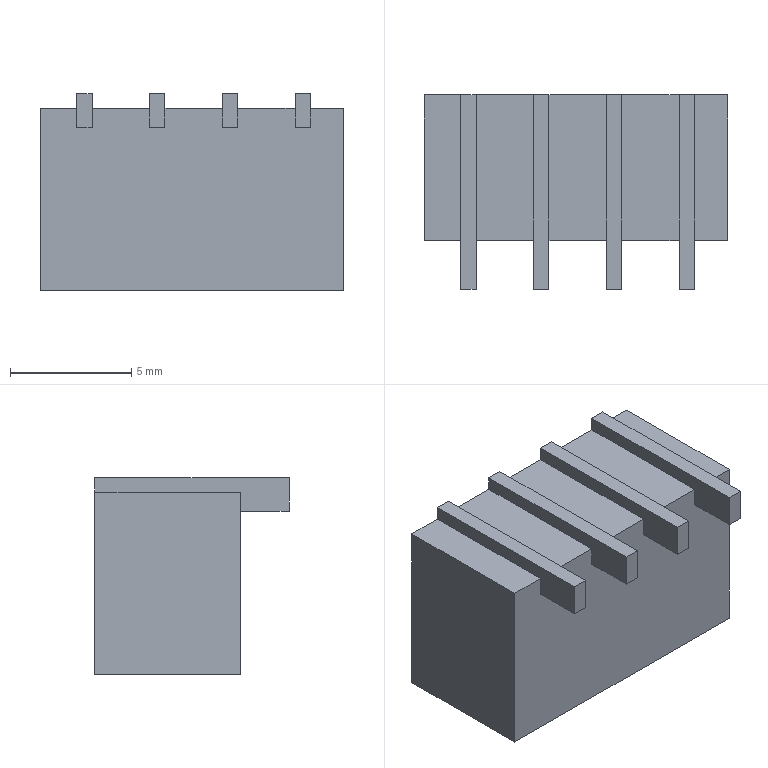Part | SolidWorks | features Boss 1, Cut 1, Extrusion 1 | 1 solid | 47 faces | box 12.5 x 8 x 8.081 mm | volume 341.66 mm3 | plane 39 | cylinder 8 | commonest cylinder face diameters 0.961 x2 1.001 x2 1.034 x2 1.165 x2
STEP:
#1=CARTESIAN_POINT('',(1.73,2.192,5.));
#2=VERTEX_POINT('',#1);
#3=CARTESIAN_POINT('',(2.731,2.192,5.));
#4=VERTEX_POINT('',#3);
#5=CARTESIAN_POINT('',(2.231,2.192,5.));
#6=DIRECTION('',(0.,0.,-1.));
#7=DIRECTION('',(-1.,0.,0.));
#8=AXIS2_PLACEMENT_3D('',#5,#6,#7);
#9=CIRCLE('',#8,0.5005);
#10=EDGE_CURVE('',#2,#4,#9,.T.);
#11=ORIENTED_EDGE('',*,*,#10,.T.);
#12=CARTESIAN_POINT('',(2.731,2.192,0.));
#13=VERTEX_POINT('',#12);
#14=CARTESIAN_POINT('',(2.731,2.192,5.));
#15=DIRECTION('',(0.,0.,-1.));
#16=VECTOR('',#15,1000.);
#17=LINE('',#14,#16);
#18=EDGE_CURVE('',#4,#13,#17,.T.);
#19=ORIENTED_EDGE('',*,*,#18,.T.);
#20=CARTESIAN_POINT('',(1.73,2.192,0.));
#21=VERTEX_POINT('',#20);
#22=CARTESIAN_POINT('',(2.231,2.192,0.));
#23=DIRECTION('',(0.,0.,-1.));
#24=DIRECTION('',(-1.,0.,0.));
#25=AXIS2_PLACEMENT_3D('',#22,#23,#24);
#26=CIRCLE('',#25,0.5005);
#27=EDGE_CURVE('',#21,#13,#26,.T.);
#28=ORIENTED_EDGE('',*,*,#27,.F.);
#29=CARTESIAN_POINT('',(1.73,2.192,5.));
#30=DIRECTION('',(0.,0.,-1.));
#31=VECTOR('',#30,1000.);
#32=LINE('',#29,#31);
#33=EDGE_CURVE('',#2,#21,#32,.T.);
#34=ORIENTED_EDGE('',*,*,#33,.F.);
#35=EDGE_LOOP('',(#11,#19,#28,#34));
#36=FACE_OUTER_BOUND('',#35,.T.);
#37=CARTESIAN_POINT('',(2.231,2.192,5.));
#38=DIRECTION('',(0.,0.,-1.));
#39=DIRECTION('',(-1.,0.,0.));
#40=AXIS2_PLACEMENT_3D('',#37,#38,#39);
#41=CYLINDRICAL_SURFACE('',#40,0.5005);
#42=ADVANCED_FACE('',(#36),#41,.T.);
#43=CARTESIAN_POINT('',(3.717,2.192,5.));
#44=VERTEX_POINT('',#43);
#45=CARTESIAN_POINT('',(4.882,2.192,5.));
#46=VERTEX_POINT('',#45);
#47=CARTESIAN_POINT('',(4.299,2.192,5.));
#48=DIRECTION('',(0.,0.,-1.));
#49=DIRECTION('',(-1.,0.,0.));
#50=AXIS2_PLACEMENT_3D('',#47,#48,#49);
#51=CIRCLE('',#50,0.5827);
#52=EDGE_CURVE('',#44,#46,#51,.T.);
#53=ORIENTED_EDGE('',*,*,#52,.T.);
#54=CARTESIAN_POINT('',(4.882,2.192,0.));
#55=VERTEX_POINT('',#54);
#56=CARTESIAN_POINT('',(4.882,2.192,5.));
#57=DIRECTION('',(0.,0.,-1.));
#58=VECTOR('',#57,1000.);
#59=LINE('',#56,#58);
#60=EDGE_CURVE('',#46,#55,#59,.T.);
#61=ORIENTED_EDGE('',*,*,#60,.T.);
#62=CARTESIAN_POINT('',(3.717,2.192,0.));
#63=VERTEX_POINT('',#62);
#64=CARTESIAN_POINT('',(4.299,2.192,0.));
#65=DIRECTION('',(0.,0.,-1.));
#66=DIRECTION('',(-1.,0.,0.));
#67=AXIS2_PLACEMENT_3D('',#64,#65,#66);
#68=CIRCLE('',#67,0.5827);
#69=EDGE_CURVE('',#63,#55,#68,.T.);
#70=ORIENTED_EDGE('',*,*,#69,.F.);
#71=CARTESIAN_POINT('',(3.717,2.192,5.));
#72=DIRECTION('',(0.,0.,-1.));
#73=VECTOR('',#72,1000.);
#74=LINE('',#71,#73);
#75=EDGE_CURVE('',#44,#63,#74,.T.);
#76=ORIENTED_EDGE('',*,*,#75,.F.);
#77=EDGE_LOOP('',(#53,#61,#70,#76));
#78=FACE_OUTER_BOUND('',#77,.T.);
#79=CARTESIAN_POINT('',(4.299,2.192,5.));
#80=DIRECTION('',(0.,0.,-1.));
#81=DIRECTION('',(-1.,0.,0.));
#82=AXIS2_PLACEMENT_3D('',#79,#80,#81);
#83=CYLINDRICAL_SURFACE('',#82,0.5827);
#84=ADVANCED_FACE('',(#78),#83,.T.);
#85=CARTESIAN_POINT('',(5.817,2.192,5.));
#86=VERTEX_POINT('',#85);
#87=CARTESIAN_POINT('',(6.852,2.192,5.));
#88=VERTEX_POINT('',#87);
#89=CARTESIAN_POINT('',(6.335,2.192,5.));
#90=DIRECTION('',(0.,0.,-1.));
#91=DIRECTION('',(-1.,0.,0.));
#92=AXIS2_PLACEMENT_3D('',#89,#90,#91);
#93=CIRCLE('',#92,0.5172);
#94=EDGE_CURVE('',#86,#88,#93,.T.);
#95=ORIENTED_EDGE('',*,*,#94,.T.);
#96=CARTESIAN_POINT('',(6.852,2.192,0.));
#97=VERTEX_POINT('',#96);
#98=CARTESIAN_POINT('',(6.852,2.192,5.));
#99=DIRECTION('',(0.,0.,-1.));
#100=VECTOR('',#99,1000.);
#101=LINE('',#98,#100);
#102=EDGE_CURVE('',#88,#97,#101,.T.);
#103=ORIENTED_EDGE('',*,*,#102,.T.);
#104=CARTESIAN_POINT('',(5.817,2.192,0.));
#105=VERTEX_POINT('',#104);
#106=CARTESIAN_POINT('',(6.335,2.192,0.));
#107=DIRECTION('',(0.,0.,-1.));
#108=DIRECTION('',(-1.,0.,0.));
#109=AXIS2_PLACEMENT_3D('',#106,#107,#108);
#110=CIRCLE('',#109,0.5172);
#111=EDGE_CURVE('',#105,#97,#110,.T.);
#112=ORIENTED_EDGE('',*,*,#111,.F.);
#113=CARTESIAN_POINT('',(5.817,2.192,5.));
#114=DIRECTION('',(0.,0.,-1.));
#115=VECTOR('',#114,1000.);
#116=LINE('',#113,#115);
#117=EDGE_CURVE('',#86,#105,#116,.T.);
#118=ORIENTED_EDGE('',*,*,#117,.F.);
#119=EDGE_LOOP('',(#95,#103,#112,#118));
#120=FACE_OUTER_BOUND('',#119,.T.);
#121=CARTESIAN_POINT('',(6.335,2.192,5.));
#122=DIRECTION('',(0.,0.,-1.));
#123=DIRECTION('',(-1.,0.,0.));
#124=AXIS2_PLACEMENT_3D('',#121,#122,#123);
#125=CYLINDRICAL_SURFACE('',#124,0.5172);
#126=ADVANCED_FACE('',(#120),#125,.T.);
#127=CARTESIAN_POINT('',(7.506,2.192,5.));
#128=VERTEX_POINT('',#127);
#129=CARTESIAN_POINT('',(8.467,2.192,5.));
#130=VERTEX_POINT('',#129);
#131=CARTESIAN_POINT('',(7.986,2.192,5.));
#132=DIRECTION('',(0.,0.,-1.));
#133=DIRECTION('',(-1.,0.,0.));
#134=AXIS2_PLACEMENT_3D('',#131,#132,#133);
#135=CIRCLE('',#134,0.4804);
#136=EDGE_CURVE('',#128,#130,#135,.T.);
#137=ORIENTED_EDGE('',*,*,#136,.T.);
#138=CARTESIAN_POINT('',(8.467,2.192,0.));
#139=VERTEX_POINT('',#138);
#140=CARTESIAN_POINT('',(8.467,2.192,5.));
#141=DIRECTION('',(0.,0.,-1.));
#142=VECTOR('',#141,1000.);
#143=LINE('',#140,#142);
#144=EDGE_CURVE('',#130,#139,#143,.T.);
#145=ORIENTED_EDGE('',*,*,#144,.T.);
#146=CARTESIAN_POINT('',(7.506,2.192,0.));
#147=VERTEX_POINT('',#146);
#148=CARTESIAN_POINT('',(7.986,2.192,0.));
#149=DIRECTION('',(0.,0.,-1.));
#150=DIRECTION('',(-1.,0.,0.));
#151=AXIS2_PLACEMENT_3D('',#148,#149,#150);
#152=CIRCLE('',#151,0.4804);
#153=EDGE_CURVE('',#147,#139,#152,.T.);
#154=ORIENTED_EDGE('',*,*,#153,.F.);
#155=CARTESIAN_POINT('',(7.506,2.192,5.));
#156=DIRECTION('',(0.,0.,-1.));
#157=VECTOR('',#156,1000.);
#158=LINE('',#155,#157);
#159=EDGE_CURVE('',#128,#147,#158,.T.);
#160=ORIENTED_EDGE('',*,*,#159,.F.);
#161=EDGE_LOOP('',(#137,#145,#154,#160));
#162=FACE_OUTER_BOUND('',#161,.T.);
#163=CARTESIAN_POINT('',(7.986,2.192,5.));
#164=DIRECTION('',(0.,0.,-1.));
#165=DIRECTION('',(-1.,0.,0.));
#166=AXIS2_PLACEMENT_3D('',#163,#164,#165);
#167=CYLINDRICAL_SURFACE('',#166,0.4804);
#168=ADVANCED_FACE('',(#162),#167,.T.);
#169=CARTESIAN_POINT('',(0.9207,-1.386,6.717));
#170=VERTEX_POINT('',#169);
#171=CARTESIAN_POINT('',(0.9207,-1.386,7.5));
#172=VERTEX_POINT('',#171);
#173=CARTESIAN_POINT('',(0.9207,-1.386,7.5));
#174=DIRECTION('',(0.,0.,1.));
#175=VECTOR('',#174,1000.);
#176=LINE('',#173,#175);
#177=EDGE_CURVE('',#170,#172,#176,.T.);
#178=ORIENTED_EDGE('',*,*,#177,.F.);
#179=CARTESIAN_POINT('',(0.2773,-1.386,6.717));
#180=VERTEX_POINT('',#179);
#181=CARTESIAN_POINT('',(11.283,-1.386,6.717));
#182=DIRECTION('',(1.,0.,0.));
#183=VECTOR('',#182,1000.);
#184=LINE('',#181,#183);
#185=EDGE_CURVE('',#180,#170,#184,.T.);
#186=ORIENTED_EDGE('',*,*,#185,.F.);
#187=CARTESIAN_POINT('',(0.2773,-1.386,7.5));
#188=VERTEX_POINT('',#187);
#189=CARTESIAN_POINT('',(0.2773,-1.386,7.5));
#190=DIRECTION('',(0.,0.,-1.));
#191=VECTOR('',#190,1000.);
#192=LINE('',#189,#191);
#193=EDGE_CURVE('',#188,#180,#192,.T.);
#194=ORIENTED_EDGE('',*,*,#193,.F.);
#195=CARTESIAN_POINT('',(-1.217,-1.386,7.5));
#196=VERTEX_POINT('',#195);
#197=CARTESIAN_POINT('',(11.283,-1.386,7.5));
#198=DIRECTION('',(1.,0.,0.));
#199=VECTOR('',#198,1000.);
#200=LINE('',#197,#199);
#201=EDGE_CURVE('',#196,#188,#200,.T.);
#202=ORIENTED_EDGE('',*,*,#201,.F.);
#203=CARTESIAN_POINT('',(-1.217,-1.386,0.));
#204=VERTEX_POINT('',#203);
#205=CARTESIAN_POINT('',(-1.217,-1.386,7.5));
#206=DIRECTION('',(0.,0.,-1.));
#207=VECTOR('',#206,1000.);
#208=LINE('',#205,#207);
#209=EDGE_CURVE('',#196,#204,#208,.T.);
#210=ORIENTED_EDGE('',*,*,#209,.T.);
#211=CARTESIAN_POINT('',(11.283,-1.386,0.));
#212=VERTEX_POINT('',#211);
#213=CARTESIAN_POINT('',(11.283,-1.386,0.));
#214=DIRECTION('',(1.,0.,0.));
#215=VECTOR('',#214,1000.);
#216=LINE('',#213,#215);
#217=EDGE_CURVE('',#204,#212,#216,.T.);
#218=ORIENTED_EDGE('',*,*,#217,.T.);
#219=CARTESIAN_POINT('',(11.283,-1.386,7.5));
#220=VERTEX_POINT('',#219);
#221=CARTESIAN_POINT('',(11.283,-1.386,7.5));
#222=DIRECTION('',(0.,0.,-1.));
#223=VECTOR('',#222,1000.);
#224=LINE('',#221,#223);
#225=EDGE_CURVE('',#220,#212,#224,.T.);
#226=ORIENTED_EDGE('',*,*,#225,.F.);
#227=CARTESIAN_POINT('',(9.921,-1.386,7.5));
#228=VERTEX_POINT('',#227);
#229=CARTESIAN_POINT('',(11.283,-1.386,7.5));
#230=DIRECTION('',(1.,0.,0.));
#231=VECTOR('',#230,1000.);
#232=LINE('',#229,#231);
#233=EDGE_CURVE('',#228,#220,#232,.T.);
#234=ORIENTED_EDGE('',*,*,#233,.F.);
#235=CARTESIAN_POINT('',(9.921,-1.386,6.717));
#236=VERTEX_POINT('',#235);
#237=CARTESIAN_POINT('',(9.921,-1.386,7.5));
#238=DIRECTION('',(0.,0.,1.));
#239=VECTOR('',#238,1000.);
#240=LINE('',#237,#239);
#241=EDGE_CURVE('',#236,#228,#240,.T.);
#242=ORIENTED_EDGE('',*,*,#241,.F.);
#243=CARTESIAN_POINT('',(9.277,-1.386,6.717));
#244=VERTEX_POINT('',#243);
#245=CARTESIAN_POINT('',(11.283,-1.386,6.717));
#246=DIRECTION('',(1.,0.,0.));
#247=VECTOR('',#246,1000.);
#248=LINE('',#245,#247);
#249=EDGE_CURVE('',#244,#236,#248,.T.);
#250=ORIENTED_EDGE('',*,*,#249,.F.);
#251=CARTESIAN_POINT('',(9.277,-1.386,7.5));
#252=VERTEX_POINT('',#251);
#253=CARTESIAN_POINT('',(9.277,-1.386,7.5));
#254=DIRECTION('',(0.,0.,-1.));
#255=VECTOR('',#254,1000.);
#256=LINE('',#253,#255);
#257=EDGE_CURVE('',#252,#244,#256,.T.);
#258=ORIENTED_EDGE('',*,*,#257,.F.);
#259=CARTESIAN_POINT('',(6.921,-1.386,7.5));
#260=VERTEX_POINT('',#259);
#261=CARTESIAN_POINT('',(11.283,-1.386,7.5));
#262=DIRECTION('',(1.,0.,0.));
#263=VECTOR('',#262,1000.);
#264=LINE('',#261,#263);
#265=EDGE_CURVE('',#260,#252,#264,.T.);
#266=ORIENTED_EDGE('',*,*,#265,.F.);
#267=CARTESIAN_POINT('',(6.921,-1.386,6.717));
#268=VERTEX_POINT('',#267);
#269=CARTESIAN_POINT('',(6.921,-1.386,7.5));
#270=DIRECTION('',(0.,0.,1.));
#271=VECTOR('',#270,1000.);
#272=LINE('',#269,#271);
#273=EDGE_CURVE('',#268,#260,#272,.T.);
#274=ORIENTED_EDGE('',*,*,#273,.F.);
#275=CARTESIAN_POINT('',(6.277,-1.386,6.717));
#276=VERTEX_POINT('',#275);
#277=CARTESIAN_POINT('',(11.283,-1.386,6.717));
#278=DIRECTION('',(1.,0.,0.));
#279=VECTOR('',#278,1000.);
#280=LINE('',#277,#279);
#281=EDGE_CURVE('',#276,#268,#280,.T.);
#282=ORIENTED_EDGE('',*,*,#281,.F.);
#283=CARTESIAN_POINT('',(6.277,-1.386,7.5));
#284=VERTEX_POINT('',#283);
#285=CARTESIAN_POINT('',(6.277,-1.386,7.5));
#286=DIRECTION('',(0.,0.,-1.));
#287=VECTOR('',#286,1000.);
#288=LINE('',#285,#287);
#289=EDGE_CURVE('',#284,#276,#288,.T.);
#290=ORIENTED_EDGE('',*,*,#289,.F.);
#291=CARTESIAN_POINT('',(3.921,-1.386,7.5));
#292=VERTEX_POINT('',#291);
#293=CARTESIAN_POINT('',(11.283,-1.386,7.5));
#294=DIRECTION('',(1.,0.,0.));
#295=VECTOR('',#294,1000.);
#296=LINE('',#293,#295);
#297=EDGE_CURVE('',#292,#284,#296,.T.);
#298=ORIENTED_EDGE('',*,*,#297,.F.);
#299=CARTESIAN_POINT('',(3.921,-1.386,6.717));
#300=VERTEX_POINT('',#299);
#301=CARTESIAN_POINT('',(3.921,-1.386,7.5));
#302=DIRECTION('',(0.,0.,1.));
#303=VECTOR('',#302,1000.);
#304=LINE('',#301,#303);
#305=EDGE_CURVE('',#300,#292,#304,.T.);
#306=ORIENTED_EDGE('',*,*,#305,.F.);
#307=CARTESIAN_POINT('',(3.277,-1.386,6.717));
#308=VERTEX_POINT('',#307);
#309=CARTESIAN_POINT('',(11.283,-1.386,6.717));
#310=DIRECTION('',(1.,0.,0.));
#311=VECTOR('',#310,1000.);
#312=LINE('',#309,#311);
#313=EDGE_CURVE('',#308,#300,#312,.T.);
#314=ORIENTED_EDGE('',*,*,#313,.F.);
#315=CARTESIAN_POINT('',(3.277,-1.386,7.5));
#316=VERTEX_POINT('',#315);
#317=CARTESIAN_POINT('',(3.277,-1.386,7.5));
#318=DIRECTION('',(0.,0.,-1.));
#319=VECTOR('',#318,1000.);
#320=LINE('',#317,#319);
#321=EDGE_CURVE('',#316,#308,#320,.T.);
#322=ORIENTED_EDGE('',*,*,#321,.F.);
#323=CARTESIAN_POINT('',(11.283,-1.386,7.5));
#324=DIRECTION('',(1.,0.,0.));
#325=VECTOR('',#324,1000.);
#326=LINE('',#323,#325);
#327=EDGE_CURVE('',#172,#316,#326,.T.);
#328=ORIENTED_EDGE('',*,*,#327,.F.);
#329=EDGE_LOOP('',(#178,#186,#194,#202,#210,#218,#226,#234,#242,#250,#258,#266,#274,#282,#290,#298,#306,#314,#322,#328));
#330=FACE_OUTER_BOUND('',#329,.T.);
#331=CARTESIAN_POINT('',(11.283,-1.386,7.5));
#332=DIRECTION('',(0.,1.,0.));
#333=DIRECTION('',(-1.,0.,0.));
#334=AXIS2_PLACEMENT_3D('',#331,#332,#333);
#335=PLANE('',#334);
#336=ADVANCED_FACE('',(#330),#335,.F.);
#337=CARTESIAN_POINT('',(3.277,4.614,7.5));
#338=VERTEX_POINT('',#337);
#339=CARTESIAN_POINT('',(0.9207,4.614,7.5));
#340=VERTEX_POINT('',#339);
#341=CARTESIAN_POINT('',(11.283,4.614,7.5));
#342=DIRECTION('',(-1.,0.,0.));
#343=VECTOR('',#342,1000.);
#344=LINE('',#341,#343);
#345=EDGE_CURVE('',#338,#340,#344,.T.);
#346=ORIENTED_EDGE('',*,*,#345,.T.);
#347=CARTESIAN_POINT('',(0.9207,4.614,7.5));
#348=DIRECTION('',(0.,-1.,0.));
#349=VECTOR('',#348,1000.);
#350=LINE('',#347,#349);
#351=EDGE_CURVE('',#340,#172,#350,.T.);
#352=ORIENTED_EDGE('',*,*,#351,.T.);
#353=ORIENTED_EDGE('',*,*,#327,.T.);
#354=CARTESIAN_POINT('',(3.277,4.614,7.5));
#355=DIRECTION('',(0.,1.,0.));
#356=VECTOR('',#355,1000.);
#357=LINE('',#354,#356);
#358=EDGE_CURVE('',#316,#338,#357,.T.);
#359=ORIENTED_EDGE('',*,*,#358,.T.);
#360=EDGE_LOOP('',(#346,#352,#353,#359));
#361=FACE_OUTER_BOUND('',#360,.T.);
#362=CARTESIAN_POINT('',(11.283,4.614,7.5));
#363=DIRECTION('',(0.,0.,1.));
#364=DIRECTION('',(1.,0.,0.));
#365=AXIS2_PLACEMENT_3D('',#362,#363,#364);
#366=PLANE('',#365);
#367=ADVANCED_FACE('',(#361),#366,.T.);
#368=ORIENTED_EDGE('',*,*,#201,.T.);
#369=CARTESIAN_POINT('',(0.2773,4.614,7.5));
#370=VERTEX_POINT('',#369);
#371=CARTESIAN_POINT('',(0.2773,4.614,7.5));
#372=DIRECTION('',(0.,1.,0.));
#373=VECTOR('',#372,1000.);
#374=LINE('',#371,#373);
#375=EDGE_CURVE('',#188,#370,#374,.T.);
#376=ORIENTED_EDGE('',*,*,#375,.T.);
#377=CARTESIAN_POINT('',(-1.217,4.614,7.5));
#378=VERTEX_POINT('',#377);
#379=CARTESIAN_POINT('',(11.283,4.614,7.5));
#380=DIRECTION('',(-1.,0.,0.));
#381=VECTOR('',#380,1000.);
#382=LINE('',#379,#381);
#383=EDGE_CURVE('',#370,#378,#382,.T.);
#384=ORIENTED_EDGE('',*,*,#383,.T.);
#385=CARTESIAN_POINT('',(-1.217,-1.386,7.5));
#386=DIRECTION('',(0.,-1.,0.));
#387=VECTOR('',#386,1000.);
#388=LINE('',#385,#387);
#389=EDGE_CURVE('',#378,#196,#388,.T.);
#390=ORIENTED_EDGE('',*,*,#389,.T.);
#391=EDGE_LOOP('',(#368,#376,#384,#390));
#392=FACE_OUTER_BOUND('',#391,.T.);
#393=CARTESIAN_POINT('',(11.283,4.614,7.5));
#394=DIRECTION('',(0.,0.,1.));
#395=DIRECTION('',(1.,0.,0.));
#396=AXIS2_PLACEMENT_3D('',#393,#394,#395);
#397=PLANE('',#396);
#398=ADVANCED_FACE('',(#392),#397,.T.);
#399=CARTESIAN_POINT('',(6.277,4.614,7.5));
#400=VERTEX_POINT('',#399);
#401=CARTESIAN_POINT('',(3.921,4.614,7.5));
#402=VERTEX_POINT('',#401);
#403=CARTESIAN_POINT('',(11.283,4.614,7.5));
#404=DIRECTION('',(-1.,0.,0.));
#405=VECTOR('',#404,1000.);
#406=LINE('',#403,#405);
#407=EDGE_CURVE('',#400,#402,#406,.T.);
#408=ORIENTED_EDGE('',*,*,#407,.T.);
#409=CARTESIAN_POINT('',(3.921,4.614,7.5));
#410=DIRECTION('',(0.,-1.,0.));
#411=VECTOR('',#410,1000.);
#412=LINE('',#409,#411);
#413=EDGE_CURVE('',#402,#292,#412,.T.);
#414=ORIENTED_EDGE('',*,*,#413,.T.);
#415=ORIENTED_EDGE('',*,*,#297,.T.);
#416=CARTESIAN_POINT('',(6.277,4.614,7.5));
#417=DIRECTION('',(0.,1.,0.));
#418=VECTOR('',#417,1000.);
#419=LINE('',#416,#418);
#420=EDGE_CURVE('',#284,#400,#419,.T.);
#421=ORIENTED_EDGE('',*,*,#420,.T.);
#422=EDGE_LOOP('',(#408,#414,#415,#421));
#423=FACE_OUTER_BOUND('',#422,.T.);
#424=CARTESIAN_POINT('',(11.283,4.614,7.5));
#425=DIRECTION('',(0.,0.,1.));
#426=DIRECTION('',(1.,0.,0.));
#427=AXIS2_PLACEMENT_3D('',#424,#425,#426);
#428=PLANE('',#427);
#429=ADVANCED_FACE('',(#423),#428,.T.);
#430=CARTESIAN_POINT('',(9.277,4.614,7.5));
#431=VERTEX_POINT('',#430);
#432=CARTESIAN_POINT('',(6.921,4.614,7.5));
#433=VERTEX_POINT('',#432);
#434=CARTESIAN_POINT('',(11.283,4.614,7.5));
#435=DIRECTION('',(-1.,0.,0.));
#436=VECTOR('',#435,1000.);
#437=LINE('',#434,#436);
#438=EDGE_CURVE('',#431,#433,#437,.T.);
#439=ORIENTED_EDGE('',*,*,#438,.T.);
#440=CARTESIAN_POINT('',(6.921,4.614,7.5));
#441=DIRECTION('',(0.,-1.,0.));
#442=VECTOR('',#441,1000.);
#443=LINE('',#440,#442);
#444=EDGE_CURVE('',#433,#260,#443,.T.);
#445=ORIENTED_EDGE('',*,*,#444,.T.);
#446=ORIENTED_EDGE('',*,*,#265,.T.);
#447=CARTESIAN_POINT('',(9.277,4.614,7.5));
#448=DIRECTION('',(0.,1.,0.));
#449=VECTOR('',#448,1000.);
#450=LINE('',#447,#449);
#451=EDGE_CURVE('',#252,#431,#450,.T.);
#452=ORIENTED_EDGE('',*,*,#451,.T.);
#453=EDGE_LOOP('',(#439,#445,#446,#452));
#454=FACE_OUTER_BOUND('',#453,.T.);
#455=CARTESIAN_POINT('',(11.283,4.614,7.5));
#456=DIRECTION('',(0.,0.,1.));
#457=DIRECTION('',(1.,0.,0.));
#458=AXIS2_PLACEMENT_3D('',#455,#456,#457);
#459=PLANE('',#458);
#460=ADVANCED_FACE('',(#454),#459,.T.);
#461=CARTESIAN_POINT('',(11.283,4.614,7.5));
#462=VERTEX_POINT('',#461);
#463=CARTESIAN_POINT('',(9.921,4.614,7.5));
#464=VERTEX_POINT('',#463);
#465=CARTESIAN_POINT('',(11.283,4.614,7.5));
#466=DIRECTION('',(-1.,0.,0.));
#467=VECTOR('',#466,1000.);
#468=LINE('',#465,#467);
#469=EDGE_CURVE('',#462,#464,#468,.T.);
#470=ORIENTED_EDGE('',*,*,#469,.T.);
#471=CARTESIAN_POINT('',(9.921,4.614,7.5));
#472=DIRECTION('',(0.,-1.,0.));
#473=VECTOR('',#472,1000.);
#474=LINE('',#471,#473);
#475=EDGE_CURVE('',#464,#228,#474,.T.);
#476=ORIENTED_EDGE('',*,*,#475,.T.);
#477=ORIENTED_EDGE('',*,*,#233,.T.);
#478=CARTESIAN_POINT('',(11.283,-1.386,7.5));
#479=DIRECTION('',(0.,1.,0.));
#480=VECTOR('',#479,1000.);
#481=LINE('',#478,#480);
#482=EDGE_CURVE('',#220,#462,#481,.T.);
#483=ORIENTED_EDGE('',*,*,#482,.T.);
#484=EDGE_LOOP('',(#470,#476,#477,#483));
#485=FACE_OUTER_BOUND('',#484,.T.);
#486=CARTESIAN_POINT('',(11.283,4.614,7.5));
#487=DIRECTION('',(0.,0.,1.));
#488=DIRECTION('',(1.,0.,0.));
#489=AXIS2_PLACEMENT_3D('',#486,#487,#488);
#490=PLANE('',#489);
#491=ADVANCED_FACE('',(#485),#490,.T.);
#492=CARTESIAN_POINT('',(11.283,4.614,0.));
#493=VERTEX_POINT('',#492);
#494=CARTESIAN_POINT('',(11.283,-1.386,0.));
#495=DIRECTION('',(0.,1.,0.));
#496=VECTOR('',#495,1000.);
#497=LINE('',#494,#496);
#498=EDGE_CURVE('',#212,#493,#497,.T.);
#499=ORIENTED_EDGE('',*,*,#498,.T.);
#500=CARTESIAN_POINT('',(11.283,4.614,7.5));
#501=DIRECTION('',(0.,0.,-1.));
#502=VECTOR('',#501,1000.);
#503=LINE('',#500,#502);
#504=EDGE_CURVE('',#462,#493,#503,.T.);
#505=ORIENTED_EDGE('',*,*,#504,.F.);
#506=ORIENTED_EDGE('',*,*,#482,.F.);
#507=ORIENTED_EDGE('',*,*,#225,.T.);
#508=EDGE_LOOP('',(#499,#505,#506,#507));
#509=FACE_OUTER_BOUND('',#508,.T.);
#510=CARTESIAN_POINT('',(11.283,-1.386,7.5));
#511=DIRECTION('',(-1.,0.,0.));
#512=DIRECTION('',(0.,0.,1.));
#513=AXIS2_PLACEMENT_3D('',#510,#511,#512);
#514=PLANE('',#513);
#515=ADVANCED_FACE('',(#509),#514,.F.);
#516=ORIENTED_EDGE('',*,*,#383,.F.);
#517=CARTESIAN_POINT('',(0.2773,4.614,8.081));
#518=VERTEX_POINT('',#517);
#519=CARTESIAN_POINT('',(0.2773,4.614,6.717));
#520=DIRECTION('',(0.,0.,-1.));
#521=VECTOR('',#520,1000.);
#522=LINE('',#519,#521);
#523=EDGE_CURVE('',#518,#370,#522,.T.);
#524=ORIENTED_EDGE('',*,*,#523,.F.);
#525=CARTESIAN_POINT('',(0.9207,4.614,8.081));
#526=VERTEX_POINT('',#525);
#527=CARTESIAN_POINT('',(0.9207,4.614,8.081));
#528=DIRECTION('',(-1.,0.,0.));
#529=VECTOR('',#528,1000.);
#530=LINE('',#527,#529);
#531=EDGE_CURVE('',#526,#518,#530,.T.);
#532=ORIENTED_EDGE('',*,*,#531,.F.);
#533=CARTESIAN_POINT('',(0.9207,4.614,6.717));
#534=DIRECTION('',(0.,0.,1.));
#535=VECTOR('',#534,1000.);
#536=LINE('',#533,#535);
#537=EDGE_CURVE('',#340,#526,#536,.T.);
#538=ORIENTED_EDGE('',*,*,#537,.F.);
#539=ORIENTED_EDGE('',*,*,#345,.F.);
#540=CARTESIAN_POINT('',(3.277,4.614,8.081));
#541=VERTEX_POINT('',#540);
#542=CARTESIAN_POINT('',(3.277,4.614,6.717));
#543=DIRECTION('',(0.,0.,-1.));
#544=VECTOR('',#543,1000.);
#545=LINE('',#542,#544);
#546=EDGE_CURVE('',#541,#338,#545,.T.);
#547=ORIENTED_EDGE('',*,*,#546,.F.);
#548=CARTESIAN_POINT('',(3.921,4.614,8.081));
#549=VERTEX_POINT('',#548);
#550=CARTESIAN_POINT('',(3.921,4.614,8.081));
#551=DIRECTION('',(-1.,0.,0.));
#552=VECTOR('',#551,1000.);
#553=LINE('',#550,#552);
#554=EDGE_CURVE('',#549,#541,#553,.T.);
#555=ORIENTED_EDGE('',*,*,#554,.F.);
#556=CARTESIAN_POINT('',(3.921,4.614,6.717));
#557=DIRECTION('',(0.,0.,1.));
#558=VECTOR('',#557,1000.);
#559=LINE('',#556,#558);
#560=EDGE_CURVE('',#402,#549,#559,.T.);
#561=ORIENTED_EDGE('',*,*,#560,.F.);
#562=ORIENTED_EDGE('',*,*,#407,.F.);
#563=CARTESIAN_POINT('',(6.277,4.614,8.081));
#564=VERTEX_POINT('',#563);
#565=CARTESIAN_POINT('',(6.277,4.614,6.717));
#566=DIRECTION('',(0.,0.,-1.));
#567=VECTOR('',#566,1000.);
#568=LINE('',#565,#567);
#569=EDGE_CURVE('',#564,#400,#568,.T.);
#570=ORIENTED_EDGE('',*,*,#569,.F.);
#571=CARTESIAN_POINT('',(6.921,4.614,8.081));
#572=VERTEX_POINT('',#571);
#573=CARTESIAN_POINT('',(6.921,4.614,8.081));
#574=DIRECTION('',(-1.,0.,0.));
#575=VECTOR('',#574,1000.);
#576=LINE('',#573,#575);
#577=EDGE_CURVE('',#572,#564,#576,.T.);
#578=ORIENTED_EDGE('',*,*,#577,.F.);
#579=CARTESIAN_POINT('',(6.921,4.614,6.717));
#580=DIRECTION('',(0.,0.,1.));
#581=VECTOR('',#580,1000.);
#582=LINE('',#579,#581);
#583=EDGE_CURVE('',#433,#572,#582,.T.);
#584=ORIENTED_EDGE('',*,*,#583,.F.);
#585=ORIENTED_EDGE('',*,*,#438,.F.);
#586=CARTESIAN_POINT('',(9.277,4.614,8.081));
#587=VERTEX_POINT('',#586);
#588=CARTESIAN_POINT('',(9.277,4.614,6.717));
#589=DIRECTION('',(0.,0.,-1.));
#590=VECTOR('',#589,1000.);
#591=LINE('',#588,#590);
#592=EDGE_CURVE('',#587,#431,#591,.T.);
#593=ORIENTED_EDGE('',*,*,#592,.F.);
#594=CARTESIAN_POINT('',(9.921,4.614,8.081));
#595=VERTEX_POINT('',#594);
#596=CARTESIAN_POINT('',(9.921,4.614,8.081));
#597=DIRECTION('',(-1.,0.,0.));
#598=VECTOR('',#597,1000.);
#599=LINE('',#596,#598);
#600=EDGE_CURVE('',#595,#587,#599,.T.);
#601=ORIENTED_EDGE('',*,*,#600,.F.);
#602=CARTESIAN_POINT('',(9.921,4.614,6.717));
#603=DIRECTION('',(0.,0.,1.));
#604=VECTOR('',#603,1000.);
#605=LINE('',#602,#604);
#606=EDGE_CURVE('',#464,#595,#605,.T.);
#607=ORIENTED_EDGE('',*,*,#606,.F.);
#608=ORIENTED_EDGE('',*,*,#469,.F.);
#609=ORIENTED_EDGE('',*,*,#504,.T.);
#610=CARTESIAN_POINT('',(-1.217,4.614,0.));
#611=VERTEX_POINT('',#610);
#612=CARTESIAN_POINT('',(11.283,4.614,0.));
#613=DIRECTION('',(-1.,0.,0.));
#614=VECTOR('',#613,1000.);
#615=LINE('',#612,#614);
#616=EDGE_CURVE('',#493,#611,#615,.T.);
#617=ORIENTED_EDGE('',*,*,#616,.T.);
#618=CARTESIAN_POINT('',(-1.217,4.614,7.5));
#619=DIRECTION('',(0.,0.,-1.));
#620=VECTOR('',#619,1000.);
#621=LINE('',#618,#620);
#622=EDGE_CURVE('',#378,#611,#621,.T.);
#623=ORIENTED_EDGE('',*,*,#622,.F.);
#624=EDGE_LOOP('',(#516,#524,#532,#538,#539,#547,#555,#561,#562,#570,#578,#584,#585,#593,#601,#607,#608,#609,#617,#623));
#625=FACE_OUTER_BOUND('',#624,.T.);
#626=CARTESIAN_POINT('',(11.283,4.614,7.5));
#627=DIRECTION('',(0.,-1.,0.));
#628=DIRECTION('',(1.,0.,0.));
#629=AXIS2_PLACEMENT_3D('',#626,#627,#628);
#630=PLANE('',#629);
#631=ADVANCED_FACE('',(#625),#630,.F.);
#632=CARTESIAN_POINT('',(-1.217,-1.386,0.));
#633=DIRECTION('',(0.,-1.,0.));
#634=VECTOR('',#633,1000.);
#635=LINE('',#632,#634);
#636=EDGE_CURVE('',#611,#204,#635,.T.);
#637=ORIENTED_EDGE('',*,*,#636,.T.);
#638=ORIENTED_EDGE('',*,*,#209,.F.);
#639=ORIENTED_EDGE('',*,*,#389,.F.);
#640=ORIENTED_EDGE('',*,*,#622,.T.);
#641=EDGE_LOOP('',(#637,#638,#639,#640));
#642=FACE_OUTER_BOUND('',#641,.T.);
#643=CARTESIAN_POINT('',(-1.217,-1.386,7.5));
#644=DIRECTION('',(1.,0.,0.));
#645=DIRECTION('',(0.,0.,-1.));
#646=AXIS2_PLACEMENT_3D('',#643,#644,#645);
#647=PLANE('',#646);
#648=ADVANCED_FACE('',(#642),#647,.F.);
#649=CARTESIAN_POINT('',(10.776,-0.509,0.));
#650=VERTEX_POINT('',#649);
#651=CARTESIAN_POINT('',(-0.5667,-0.509,0.));
#652=VERTEX_POINT('',#651);
#653=CARTESIAN_POINT('',(10.776,-0.509,0.));
#654=DIRECTION('',(-1.,0.,0.));
#655=VECTOR('',#654,1000.);
#656=LINE('',#653,#655);
#657=EDGE_CURVE('',#650,#652,#656,.T.);
#658=ORIENTED_EDGE('',*,*,#657,.F.);
#659=CARTESIAN_POINT('',(10.776,3.968,0.));
#660=VERTEX_POINT('',#659);
#661=CARTESIAN_POINT('',(10.776,-0.509,0.));
#662=DIRECTION('',(0.,-1.,0.));
#663=VECTOR('',#662,1000.);
#664=LINE('',#661,#663);
#665=EDGE_CURVE('',#660,#650,#664,.T.);
#666=ORIENTED_EDGE('',*,*,#665,.F.);
#667=CARTESIAN_POINT('',(-0.5667,3.968,0.));
#668=VERTEX_POINT('',#667);
#669=CARTESIAN_POINT('',(10.776,3.968,0.));
#670=DIRECTION('',(1.,0.,0.));
#671=VECTOR('',#670,1000.);
#672=LINE('',#669,#671);
#673=EDGE_CURVE('',#668,#660,#672,.T.);
#674=ORIENTED_EDGE('',*,*,#673,.F.);
#675=CARTESIAN_POINT('',(-0.5667,-0.509,0.));
#676=DIRECTION('',(0.,1.,0.));
#677=VECTOR('',#676,1000.);
#678=LINE('',#675,#677);
#679=EDGE_CURVE('',#652,#668,#678,.T.);
#680=ORIENTED_EDGE('',*,*,#679,.F.);
#681=EDGE_LOOP('',(#658,#666,#674,#680));
#682=FACE_BOUND('',#681,.T.);
#683=ORIENTED_EDGE('',*,*,#498,.F.);
#684=ORIENTED_EDGE('',*,*,#217,.F.);
#685=ORIENTED_EDGE('',*,*,#636,.F.);
#686=ORIENTED_EDGE('',*,*,#616,.F.);
#687=EDGE_LOOP('',(#683,#684,#685,#686));
#688=FACE_OUTER_BOUND('',#687,.T.);
#689=CARTESIAN_POINT('',(11.283,4.614,0.));
#690=DIRECTION('',(0.,0.,1.));
#691=DIRECTION('',(1.,0.,0.));
#692=AXIS2_PLACEMENT_3D('',#689,#690,#691);
#693=PLANE('',#692);
#694=ADVANCED_FACE('',(#682,#688),#693,.F.);
#695=ORIENTED_EDGE('',*,*,#665,.T.);
#696=CARTESIAN_POINT('',(10.776,-0.509,5.));
#697=VERTEX_POINT('',#696);
#698=CARTESIAN_POINT('',(10.776,-0.509,5.));
#699=DIRECTION('',(0.,0.,-1.));
#700=VECTOR('',#699,1000.);
#701=LINE('',#698,#700);
#702=EDGE_CURVE('',#697,#650,#701,.T.);
#703=ORIENTED_EDGE('',*,*,#702,.F.);
#704=CARTESIAN_POINT('',(10.776,3.968,5.));
#705=VERTEX_POINT('',#704);
#706=CARTESIAN_POINT('',(10.776,-0.509,5.));
#707=DIRECTION('',(0.,-1.,0.));
#708=VECTOR('',#707,1000.);
#709=LINE('',#706,#708);
#710=EDGE_CURVE('',#705,#697,#709,.T.);
#711=ORIENTED_EDGE('',*,*,#710,.F.);
#712=CARTESIAN_POINT('',(10.776,3.968,5.));
#713=DIRECTION('',(0.,0.,-1.));
#714=VECTOR('',#713,1000.);
#715=LINE('',#712,#714);
#716=EDGE_CURVE('',#705,#660,#715,.T.);
#717=ORIENTED_EDGE('',*,*,#716,.T.);
#718=EDGE_LOOP('',(#695,#703,#711,#717));
#719=FACE_OUTER_BOUND('',#718,.T.);
#720=CARTESIAN_POINT('',(10.776,-0.509,5.));
#721=DIRECTION('',(1.,0.,0.));
#722=DIRECTION('',(0.,0.,-1.));
#723=AXIS2_PLACEMENT_3D('',#720,#721,#722);
#724=PLANE('',#723);
#725=ADVANCED_FACE('',(#719),#724,.F.);
#726=ORIENTED_EDGE('',*,*,#673,.T.);
#727=ORIENTED_EDGE('',*,*,#716,.F.);
#728=CARTESIAN_POINT('',(-0.5667,3.968,5.));
#729=VERTEX_POINT('',#728);
#730=CARTESIAN_POINT('',(10.776,3.968,5.));
#731=DIRECTION('',(1.,0.,0.));
#732=VECTOR('',#731,1000.);
#733=LINE('',#730,#732);
#734=EDGE_CURVE('',#729,#705,#733,.T.);
#735=ORIENTED_EDGE('',*,*,#734,.F.);
#736=CARTESIAN_POINT('',(-0.5667,3.968,5.));
#737=DIRECTION('',(0.,0.,-1.));
#738=VECTOR('',#737,1000.);
#739=LINE('',#736,#738);
#740=EDGE_CURVE('',#729,#668,#739,.T.);
#741=ORIENTED_EDGE('',*,*,#740,.T.);
#742=EDGE_LOOP('',(#726,#727,#735,#741));
#743=FACE_OUTER_BOUND('',#742,.T.);
#744=CARTESIAN_POINT('',(10.776,3.968,5.));
#745=DIRECTION('',(0.,1.,0.));
#746=DIRECTION('',(0.,0.,1.));
#747=AXIS2_PLACEMENT_3D('',#744,#745,#746);
#748=PLANE('',#747);
#749=ADVANCED_FACE('',(#743),#748,.F.);
#750=ORIENTED_EDGE('',*,*,#679,.T.);
#751=ORIENTED_EDGE('',*,*,#740,.F.);
#752=CARTESIAN_POINT('',(-0.5667,-0.509,5.));
#753=VERTEX_POINT('',#752);
#754=CARTESIAN_POINT('',(-0.5667,-0.509,5.));
#755=DIRECTION('',(0.,1.,0.));
#756=VECTOR('',#755,1000.);
#757=LINE('',#754,#756);
#758=EDGE_CURVE('',#753,#729,#757,.T.);
#759=ORIENTED_EDGE('',*,*,#758,.F.);
#760=CARTESIAN_POINT('',(-0.5667,-0.509,5.));
#761=DIRECTION('',(0.,0.,-1.));
#762=VECTOR('',#761,1000.);
#763=LINE('',#760,#762);
#764=EDGE_CURVE('',#753,#652,#763,.T.);
#765=ORIENTED_EDGE('',*,*,#764,.T.);
#766=EDGE_LOOP('',(#750,#751,#759,#765));
#767=FACE_OUTER_BOUND('',#766,.T.);
#768=CARTESIAN_POINT('',(-0.5667,-0.509,5.));
#769=DIRECTION('',(-1.,0.,0.));
#770=DIRECTION('',(0.,0.,1.));
#771=AXIS2_PLACEMENT_3D('',#768,#769,#770);
#772=PLANE('',#771);
#773=ADVANCED_FACE('',(#767),#772,.F.);
#774=ORIENTED_EDGE('',*,*,#657,.T.);
#775=ORIENTED_EDGE('',*,*,#764,.F.);
#776=CARTESIAN_POINT('',(10.776,-0.509,5.));
#777=DIRECTION('',(-1.,0.,0.));
#778=VECTOR('',#777,1000.);
#779=LINE('',#776,#778);
#780=EDGE_CURVE('',#697,#753,#779,.T.);
#781=ORIENTED_EDGE('',*,*,#780,.F.);
#782=ORIENTED_EDGE('',*,*,#702,.T.);
#783=EDGE_LOOP('',(#774,#775,#781,#782));
#784=FACE_OUTER_BOUND('',#783,.T.);
#785=CARTESIAN_POINT('',(10.776,-0.509,5.));
#786=DIRECTION('',(0.,-1.,0.));
#787=DIRECTION('',(0.,0.,-1.));
#788=AXIS2_PLACEMENT_3D('',#785,#786,#787);
#789=PLANE('',#788);
#790=ADVANCED_FACE('',(#784),#789,.F.);
#791=ORIENTED_EDGE('',*,*,#10,.F.);
#792=CARTESIAN_POINT('',(2.231,2.192,5.));
#793=DIRECTION('',(0.,0.,-1.));
#794=DIRECTION('',(-1.,0.,0.));
#795=AXIS2_PLACEMENT_3D('',#792,#793,#794);
#796=CIRCLE('',#795,0.5005);
#797=EDGE_CURVE('',#4,#2,#796,.T.);
#798=ORIENTED_EDGE('',*,*,#797,.F.);
#799=EDGE_LOOP('',(#791,#798));
#800=FACE_BOUND('',#799,.T.);
#801=ORIENTED_EDGE('',*,*,#52,.F.);
#802=CARTESIAN_POINT('',(4.299,2.192,5.));
#803=DIRECTION('',(0.,0.,-1.));
#804=DIRECTION('',(-1.,0.,0.));
#805=AXIS2_PLACEMENT_3D('',#802,#803,#804);
#806=CIRCLE('',#805,0.5827);
#807=EDGE_CURVE('',#46,#44,#806,.T.);
#808=ORIENTED_EDGE('',*,*,#807,.F.);
#809=EDGE_LOOP('',(#801,#808));
#810=FACE_BOUND('',#809,.T.);
#811=ORIENTED_EDGE('',*,*,#94,.F.);
#812=CARTESIAN_POINT('',(6.335,2.192,5.));
#813=DIRECTION('',(0.,0.,-1.));
#814=DIRECTION('',(-1.,0.,0.));
#815=AXIS2_PLACEMENT_3D('',#812,#813,#814);
#816=CIRCLE('',#815,0.5172);
#817=EDGE_CURVE('',#88,#86,#816,.T.);
#818=ORIENTED_EDGE('',*,*,#817,.F.);
#819=EDGE_LOOP('',(#811,#818));
#820=FACE_BOUND('',#819,.T.);
#821=ORIENTED_EDGE('',*,*,#136,.F.);
#822=CARTESIAN_POINT('',(7.986,2.192,5.));
#823=DIRECTION('',(0.,0.,-1.));
#824=DIRECTION('',(-1.,0.,0.));
#825=AXIS2_PLACEMENT_3D('',#822,#823,#824);
#826=CIRCLE('',#825,0.4804);
#827=EDGE_CURVE('',#130,#128,#826,.T.);
#828=ORIENTED_EDGE('',*,*,#827,.F.);
#829=EDGE_LOOP('',(#821,#828));
#830=FACE_BOUND('',#829,.T.);
#831=ORIENTED_EDGE('',*,*,#710,.T.);
#832=ORIENTED_EDGE('',*,*,#780,.T.);
#833=ORIENTED_EDGE('',*,*,#758,.T.);
#834=ORIENTED_EDGE('',*,*,#734,.T.);
#835=EDGE_LOOP('',(#831,#832,#833,#834));
#836=FACE_OUTER_BOUND('',#835,.T.);
#837=CARTESIAN_POINT('',(10.776,3.968,5.));
#838=DIRECTION('',(0.,0.,1.));
#839=DIRECTION('',(1.,0.,0.));
#840=AXIS2_PLACEMENT_3D('',#837,#838,#839);
#841=PLANE('',#840);
#842=ADVANCED_FACE('',(#800,#810,#820,#830,#836),#841,.F.);
#843=ORIENTED_EDGE('',*,*,#144,.F.);
#844=ORIENTED_EDGE('',*,*,#827,.T.);
#845=ORIENTED_EDGE('',*,*,#159,.T.);
#846=CARTESIAN_POINT('',(7.986,2.192,0.));
#847=DIRECTION('',(0.,0.,-1.));
#848=DIRECTION('',(-1.,0.,0.));
#849=AXIS2_PLACEMENT_3D('',#846,#847,#848);
#850=CIRCLE('',#849,0.4804);
#851=EDGE_CURVE('',#139,#147,#850,.T.);
#852=ORIENTED_EDGE('',*,*,#851,.F.);
#853=EDGE_LOOP('',(#843,#844,#845,#852));
#854=FACE_OUTER_BOUND('',#853,.T.);
#855=CARTESIAN_POINT('',(7.986,2.192,5.));
#856=DIRECTION('',(0.,0.,-1.));
#857=DIRECTION('',(-1.,0.,0.));
#858=AXIS2_PLACEMENT_3D('',#855,#856,#857);
#859=CYLINDRICAL_SURFACE('',#858,0.4804);
#860=ADVANCED_FACE('',(#854),#859,.T.);
#861=ORIENTED_EDGE('',*,*,#102,.F.);
#862=ORIENTED_EDGE('',*,*,#817,.T.);
#863=ORIENTED_EDGE('',*,*,#117,.T.);
#864=CARTESIAN_POINT('',(6.335,2.192,0.));
#865=DIRECTION('',(0.,0.,-1.));
#866=DIRECTION('',(-1.,0.,0.));
#867=AXIS2_PLACEMENT_3D('',#864,#865,#866);
#868=CIRCLE('',#867,0.5172);
#869=EDGE_CURVE('',#97,#105,#868,.T.);
#870=ORIENTED_EDGE('',*,*,#869,.F.);
#871=EDGE_LOOP('',(#861,#862,#863,#870));
#872=FACE_OUTER_BOUND('',#871,.T.);
#873=CARTESIAN_POINT('',(6.335,2.192,5.));
#874=DIRECTION('',(0.,0.,-1.));
#875=DIRECTION('',(-1.,0.,0.));
#876=AXIS2_PLACEMENT_3D('',#873,#874,#875);
#877=CYLINDRICAL_SURFACE('',#876,0.5172);
#878=ADVANCED_FACE('',(#872),#877,.T.);
#879=ORIENTED_EDGE('',*,*,#60,.F.);
#880=ORIENTED_EDGE('',*,*,#807,.T.);
#881=ORIENTED_EDGE('',*,*,#75,.T.);
#882=CARTESIAN_POINT('',(4.299,2.192,0.));
#883=DIRECTION('',(0.,0.,-1.));
#884=DIRECTION('',(-1.,0.,0.));
#885=AXIS2_PLACEMENT_3D('',#882,#883,#884);
#886=CIRCLE('',#885,0.5827);
#887=EDGE_CURVE('',#55,#63,#886,.T.);
#888=ORIENTED_EDGE('',*,*,#887,.F.);
#889=EDGE_LOOP('',(#879,#880,#881,#888));
#890=FACE_OUTER_BOUND('',#889,.T.);
#891=CARTESIAN_POINT('',(4.299,2.192,5.));
#892=DIRECTION('',(0.,0.,-1.));
#893=DIRECTION('',(-1.,0.,0.));
#894=AXIS2_PLACEMENT_3D('',#891,#892,#893);
#895=CYLINDRICAL_SURFACE('',#894,0.5827);
#896=ADVANCED_FACE('',(#890),#895,.T.);
#897=ORIENTED_EDGE('',*,*,#18,.F.);
#898=ORIENTED_EDGE('',*,*,#797,.T.);
#899=ORIENTED_EDGE('',*,*,#33,.T.);
#900=CARTESIAN_POINT('',(2.231,2.192,0.));
#901=DIRECTION('',(0.,0.,-1.));
#902=DIRECTION('',(-1.,0.,0.));
#903=AXIS2_PLACEMENT_3D('',#900,#901,#902);
#904=CIRCLE('',#903,0.5005);
#905=EDGE_CURVE('',#13,#21,#904,.T.);
#906=ORIENTED_EDGE('',*,*,#905,.F.);
#907=EDGE_LOOP('',(#897,#898,#899,#906));
#908=FACE_OUTER_BOUND('',#907,.T.);
#909=CARTESIAN_POINT('',(2.231,2.192,5.));
#910=DIRECTION('',(0.,0.,-1.));
#911=DIRECTION('',(-1.,0.,0.));
#912=AXIS2_PLACEMENT_3D('',#909,#910,#911);
#913=CYLINDRICAL_SURFACE('',#912,0.5005);
#914=ADVANCED_FACE('',(#908),#913,.T.);
#915=ORIENTED_EDGE('',*,*,#69,.T.);
#916=ORIENTED_EDGE('',*,*,#887,.T.);
#917=EDGE_LOOP('',(#915,#916));
#918=FACE_OUTER_BOUND('',#917,.T.);
#919=CARTESIAN_POINT('',(11.283,4.614,0.));
#920=DIRECTION('',(0.,0.,1.));
#921=DIRECTION('',(1.,0.,0.));
#922=AXIS2_PLACEMENT_3D('',#919,#920,#921);
#923=PLANE('',#922);
#924=ADVANCED_FACE('',(#918),#923,.F.);
#925=ORIENTED_EDGE('',*,*,#111,.T.);
#926=ORIENTED_EDGE('',*,*,#869,.T.);
#927=EDGE_LOOP('',(#925,#926));
#928=FACE_OUTER_BOUND('',#927,.T.);
#929=CARTESIAN_POINT('',(11.283,4.614,0.));
#930=DIRECTION('',(0.,0.,1.));
#931=DIRECTION('',(1.,0.,0.));
#932=AXIS2_PLACEMENT_3D('',#929,#930,#931);
#933=PLANE('',#932);
#934=ADVANCED_FACE('',(#928),#933,.F.);
#935=ORIENTED_EDGE('',*,*,#153,.T.);
#936=ORIENTED_EDGE('',*,*,#851,.T.);
#937=EDGE_LOOP('',(#935,#936));
#938=FACE_OUTER_BOUND('',#937,.T.);
#939=CARTESIAN_POINT('',(11.283,4.614,0.));
#940=DIRECTION('',(0.,0.,1.));
#941=DIRECTION('',(1.,0.,0.));
#942=AXIS2_PLACEMENT_3D('',#939,#940,#941);
#943=PLANE('',#942);
#944=ADVANCED_FACE('',(#938),#943,.F.);
#945=ORIENTED_EDGE('',*,*,#27,.T.);
#946=ORIENTED_EDGE('',*,*,#905,.T.);
#947=EDGE_LOOP('',(#945,#946));
#948=FACE_OUTER_BOUND('',#947,.T.);
#949=CARTESIAN_POINT('',(11.283,4.614,0.));
#950=DIRECTION('',(0.,0.,1.));
#951=DIRECTION('',(1.,0.,0.));
#952=AXIS2_PLACEMENT_3D('',#949,#950,#951);
#953=PLANE('',#952);
#954=ADVANCED_FACE('',(#948),#953,.F.);
#955=CARTESIAN_POINT('',(9.277,-3.386,6.717));
#956=VERTEX_POINT('',#955);
#957=CARTESIAN_POINT('',(9.277,-3.386,6.717));
#958=DIRECTION('',(0.,1.,0.));
#959=VECTOR('',#958,1000.);
#960=LINE('',#957,#959);
#961=EDGE_CURVE('',#956,#244,#960,.T.);
#962=ORIENTED_EDGE('',*,*,#961,.T.);
#963=ORIENTED_EDGE('',*,*,#249,.T.);
#964=CARTESIAN_POINT('',(9.921,-3.386,6.717));
#965=VERTEX_POINT('',#964);
#966=CARTESIAN_POINT('',(9.921,-3.386,6.717));
#967=DIRECTION('',(0.,1.,0.));
#968=VECTOR('',#967,1000.);
#969=LINE('',#966,#968);
#970=EDGE_CURVE('',#965,#236,#969,.T.);
#971=ORIENTED_EDGE('',*,*,#970,.F.);
#972=CARTESIAN_POINT('',(9.921,-3.386,6.717));
#973=DIRECTION('',(1.,0.,0.));
#974=VECTOR('',#973,1000.);
#975=LINE('',#972,#974);
#976=EDGE_CURVE('',#956,#965,#975,.T.);
#977=ORIENTED_EDGE('',*,*,#976,.F.);
#978=EDGE_LOOP('',(#962,#963,#971,#977));
#979=FACE_OUTER_BOUND('',#978,.T.);
#980=CARTESIAN_POINT('',(9.921,-3.386,6.717));
#981=DIRECTION('',(0.,0.,1.));
#982=DIRECTION('',(1.,0.,0.));
#983=AXIS2_PLACEMENT_3D('',#980,#981,#982);
#984=PLANE('',#983);
#985=ADVANCED_FACE('',(#979),#984,.F.);
#986=ORIENTED_EDGE('',*,*,#970,.T.);
#987=ORIENTED_EDGE('',*,*,#241,.T.);
#988=ORIENTED_EDGE('',*,*,#475,.F.);
#989=ORIENTED_EDGE('',*,*,#606,.T.);
#990=CARTESIAN_POINT('',(9.921,-3.386,8.081));
#991=VERTEX_POINT('',#990);
#992=CARTESIAN_POINT('',(9.921,-3.386,8.081));
#993=DIRECTION('',(0.,1.,0.));
#994=VECTOR('',#993,1000.);
#995=LINE('',#992,#994);
#996=EDGE_CURVE('',#991,#595,#995,.T.);
#997=ORIENTED_EDGE('',*,*,#996,.F.);
#998=CARTESIAN_POINT('',(9.921,-3.386,6.717));
#999=DIRECTION('',(0.,0.,1.));
#1000=VECTOR('',#999,1000.);
#1001=LINE('',#998,#1000);
#1002=EDGE_CURVE('',#965,#991,#1001,.T.);
#1003=ORIENTED_EDGE('',*,*,#1002,.F.);
#1004=EDGE_LOOP('',(#986,#987,#988,#989,#997,#1003));
#1005=FACE_OUTER_BOUND('',#1004,.T.);
#1006=CARTESIAN_POINT('',(9.921,-3.386,6.717));
#1007=DIRECTION('',(-1.,0.,0.));
#1008=DIRECTION('',(0.,-1.,0.));
#1009=AXIS2_PLACEMENT_3D('',#1006,#1007,#1008);
#1010=PLANE('',#1009);
#1011=ADVANCED_FACE('',(#1005),#1010,.F.);
#1012=ORIENTED_EDGE('',*,*,#451,.F.);
#1013=ORIENTED_EDGE('',*,*,#257,.T.);
#1014=ORIENTED_EDGE('',*,*,#961,.F.);
#1015=CARTESIAN_POINT('',(9.277,-3.386,8.081));
#1016=VERTEX_POINT('',#1015);
#1017=CARTESIAN_POINT('',(9.277,-3.386,6.717));
#1018=DIRECTION('',(0.,0.,-1.));
#1019=VECTOR('',#1018,1000.);
#1020=LINE('',#1017,#1019);
#1021=EDGE_CURVE('',#1016,#956,#1020,.T.);
#1022=ORIENTED_EDGE('',*,*,#1021,.F.);
#1023=CARTESIAN_POINT('',(9.277,-3.386,8.081));
#1024=DIRECTION('',(0.,1.,0.));
#1025=VECTOR('',#1024,1000.);
#1026=LINE('',#1023,#1025);
#1027=EDGE_CURVE('',#1016,#587,#1026,.T.);
#1028=ORIENTED_EDGE('',*,*,#1027,.T.);
#1029=ORIENTED_EDGE('',*,*,#592,.T.);
#1030=EDGE_LOOP('',(#1012,#1013,#1014,#1022,#1028,#1029));
#1031=FACE_OUTER_BOUND('',#1030,.T.);
#1032=CARTESIAN_POINT('',(9.277,-3.386,6.717));
#1033=DIRECTION('',(1.,0.,0.));
#1034=DIRECTION('',(0.,1.,0.));
#1035=AXIS2_PLACEMENT_3D('',#1032,#1033,#1034);
#1036=PLANE('',#1035);
#1037=ADVANCED_FACE('',(#1031),#1036,.F.);
#1038=ORIENTED_EDGE('',*,*,#600,.T.);
#1039=ORIENTED_EDGE('',*,*,#1027,.F.);
#1040=CARTESIAN_POINT('',(9.921,-3.386,8.081));
#1041=DIRECTION('',(-1.,0.,0.));
#1042=VECTOR('',#1041,1000.);
#1043=LINE('',#1040,#1042);
#1044=EDGE_CURVE('',#991,#1016,#1043,.T.);
#1045=ORIENTED_EDGE('',*,*,#1044,.F.);
#1046=ORIENTED_EDGE('',*,*,#996,.T.);
#1047=EDGE_LOOP('',(#1038,#1039,#1045,#1046));
#1048=FACE_OUTER_BOUND('',#1047,.T.);
#1049=CARTESIAN_POINT('',(9.921,-3.386,8.081));
#1050=DIRECTION('',(0.,0.,-1.));
#1051=DIRECTION('',(-1.,0.,0.));
#1052=AXIS2_PLACEMENT_3D('',#1049,#1050,#1051);
#1053=PLANE('',#1052);
#1054=ADVANCED_FACE('',(#1048),#1053,.F.);
#1055=ORIENTED_EDGE('',*,*,#1002,.T.);
#1056=ORIENTED_EDGE('',*,*,#1044,.T.);
#1057=ORIENTED_EDGE('',*,*,#1021,.T.);
#1058=ORIENTED_EDGE('',*,*,#976,.T.);
#1059=EDGE_LOOP('',(#1055,#1056,#1057,#1058));
#1060=FACE_OUTER_BOUND('',#1059,.T.);
#1061=CARTESIAN_POINT('',(9.921,-3.386,8.081));
#1062=DIRECTION('',(0.,-1.,0.));
#1063=DIRECTION('',(0.,0.,-1.));
#1064=AXIS2_PLACEMENT_3D('',#1061,#1062,#1063);
#1065=PLANE('',#1064);
#1066=ADVANCED_FACE('',(#1060),#1065,.T.);
#1067=CARTESIAN_POINT('',(6.921,-3.386,6.717));
#1068=VERTEX_POINT('',#1067);
#1069=CARTESIAN_POINT('',(6.921,-3.386,6.717));
#1070=DIRECTION('',(0.,1.,0.));
#1071=VECTOR('',#1070,1000.);
#1072=LINE('',#1069,#1071);
#1073=EDGE_CURVE('',#1068,#268,#1072,.T.);
#1074=ORIENTED_EDGE('',*,*,#1073,.T.);
#1075=ORIENTED_EDGE('',*,*,#273,.T.);
#1076=ORIENTED_EDGE('',*,*,#444,.F.);
#1077=ORIENTED_EDGE('',*,*,#583,.T.);
#1078=CARTESIAN_POINT('',(6.921,-3.386,8.081));
#1079=VERTEX_POINT('',#1078);
#1080=CARTESIAN_POINT('',(6.921,-3.386,8.081));
#1081=DIRECTION('',(0.,1.,0.));
#1082=VECTOR('',#1081,1000.);
#1083=LINE('',#1080,#1082);
#1084=EDGE_CURVE('',#1079,#572,#1083,.T.);
#1085=ORIENTED_EDGE('',*,*,#1084,.F.);
#1086=CARTESIAN_POINT('',(6.921,-3.386,6.717));
#1087=DIRECTION('',(0.,0.,1.));
#1088=VECTOR('',#1087,1000.);
#1089=LINE('',#1086,#1088);
#1090=EDGE_CURVE('',#1068,#1079,#1089,.T.);
#1091=ORIENTED_EDGE('',*,*,#1090,.F.);
#1092=EDGE_LOOP('',(#1074,#1075,#1076,#1077,#1085,#1091));
#1093=FACE_OUTER_BOUND('',#1092,.T.);
#1094=CARTESIAN_POINT('',(6.921,-3.386,6.717));
#1095=DIRECTION('',(-1.,0.,0.));
#1096=DIRECTION('',(0.,-1.,0.));
#1097=AXIS2_PLACEMENT_3D('',#1094,#1095,#1096);
#1098=PLANE('',#1097);
#1099=ADVANCED_FACE('',(#1093),#1098,.F.);
#1100=ORIENTED_EDGE('',*,*,#420,.F.);
#1101=ORIENTED_EDGE('',*,*,#289,.T.);
#1102=CARTESIAN_POINT('',(6.277,-3.386,6.717));
#1103=VERTEX_POINT('',#1102);
#1104=CARTESIAN_POINT('',(6.277,-3.386,6.717));
#1105=DIRECTION('',(0.,1.,0.));
#1106=VECTOR('',#1105,1000.);
#1107=LINE('',#1104,#1106);
#1108=EDGE_CURVE('',#1103,#276,#1107,.T.);
#1109=ORIENTED_EDGE('',*,*,#1108,.F.);
#1110=CARTESIAN_POINT('',(6.277,-3.386,8.081));
#1111=VERTEX_POINT('',#1110);
#1112=CARTESIAN_POINT('',(6.277,-3.386,6.717));
#1113=DIRECTION('',(0.,0.,-1.));
#1114=VECTOR('',#1113,1000.);
#1115=LINE('',#1112,#1114);
#1116=EDGE_CURVE('',#1111,#1103,#1115,.T.);
#1117=ORIENTED_EDGE('',*,*,#1116,.F.);
#1118=CARTESIAN_POINT('',(6.277,-3.386,8.081));
#1119=DIRECTION('',(0.,1.,0.));
#1120=VECTOR('',#1119,1000.);
#1121=LINE('',#1118,#1120);
#1122=EDGE_CURVE('',#1111,#564,#1121,.T.);
#1123=ORIENTED_EDGE('',*,*,#1122,.T.);
#1124=ORIENTED_EDGE('',*,*,#569,.T.);
#1125=EDGE_LOOP('',(#1100,#1101,#1109,#1117,#1123,#1124));
#1126=FACE_OUTER_BOUND('',#1125,.T.);
#1127=CARTESIAN_POINT('',(6.277,-3.386,6.717));
#1128=DIRECTION('',(1.,0.,0.));
#1129=DIRECTION('',(0.,1.,0.));
#1130=AXIS2_PLACEMENT_3D('',#1127,#1128,#1129);
#1131=PLANE('',#1130);
#1132=ADVANCED_FACE('',(#1126),#1131,.F.);
#1133=ORIENTED_EDGE('',*,*,#1108,.T.);
#1134=ORIENTED_EDGE('',*,*,#281,.T.);
#1135=ORIENTED_EDGE('',*,*,#1073,.F.);
#1136=CARTESIAN_POINT('',(6.921,-3.386,6.717));
#1137=DIRECTION('',(1.,0.,0.));
#1138=VECTOR('',#1137,1000.);
#1139=LINE('',#1136,#1138);
#1140=EDGE_CURVE('',#1103,#1068,#1139,.T.);
#1141=ORIENTED_EDGE('',*,*,#1140,.F.);
#1142=EDGE_LOOP('',(#1133,#1134,#1135,#1141));
#1143=FACE_OUTER_BOUND('',#1142,.T.);
#1144=CARTESIAN_POINT('',(6.921,-3.386,6.717));
#1145=DIRECTION('',(0.,0.,1.));
#1146=DIRECTION('',(1.,0.,0.));
#1147=AXIS2_PLACEMENT_3D('',#1144,#1145,#1146);
#1148=PLANE('',#1147);
#1149=ADVANCED_FACE('',(#1143),#1148,.F.);
#1150=ORIENTED_EDGE('',*,*,#577,.T.);
#1151=ORIENTED_EDGE('',*,*,#1122,.F.);
#1152=CARTESIAN_POINT('',(6.921,-3.386,8.081));
#1153=DIRECTION('',(-1.,0.,0.));
#1154=VECTOR('',#1153,1000.);
#1155=LINE('',#1152,#1154);
#1156=EDGE_CURVE('',#1079,#1111,#1155,.T.);
#1157=ORIENTED_EDGE('',*,*,#1156,.F.);
#1158=ORIENTED_EDGE('',*,*,#1084,.T.);
#1159=EDGE_LOOP('',(#1150,#1151,#1157,#1158));
#1160=FACE_OUTER_BOUND('',#1159,.T.);
#1161=CARTESIAN_POINT('',(6.921,-3.386,8.081));
#1162=DIRECTION('',(0.,0.,-1.));
#1163=DIRECTION('',(-1.,0.,0.));
#1164=AXIS2_PLACEMENT_3D('',#1161,#1162,#1163);
#1165=PLANE('',#1164);
#1166=ADVANCED_FACE('',(#1160),#1165,.F.);
#1167=ORIENTED_EDGE('',*,*,#1090,.T.);
#1168=ORIENTED_EDGE('',*,*,#1156,.T.);
#1169=ORIENTED_EDGE('',*,*,#1116,.T.);
#1170=ORIENTED_EDGE('',*,*,#1140,.T.);
#1171=EDGE_LOOP('',(#1167,#1168,#1169,#1170));
#1172=FACE_OUTER_BOUND('',#1171,.T.);
#1173=CARTESIAN_POINT('',(6.921,-3.386,8.081));
#1174=DIRECTION('',(0.,-1.,0.));
#1175=DIRECTION('',(0.,0.,-1.));
#1176=AXIS2_PLACEMENT_3D('',#1173,#1174,#1175);
#1177=PLANE('',#1176);
#1178=ADVANCED_FACE('',(#1172),#1177,.T.);
#1179=CARTESIAN_POINT('',(3.921,-3.386,6.717));
#1180=VERTEX_POINT('',#1179);
#1181=CARTESIAN_POINT('',(3.921,-3.386,6.717));
#1182=DIRECTION('',(0.,1.,0.));
#1183=VECTOR('',#1182,1000.);
#1184=LINE('',#1181,#1183);
#1185=EDGE_CURVE('',#1180,#300,#1184,.T.);
#1186=ORIENTED_EDGE('',*,*,#1185,.T.);
#1187=ORIENTED_EDGE('',*,*,#305,.T.);
#1188=ORIENTED_EDGE('',*,*,#413,.F.);
#1189=ORIENTED_EDGE('',*,*,#560,.T.);
#1190=CARTESIAN_POINT('',(3.921,-3.386,8.081));
#1191=VERTEX_POINT('',#1190);
#1192=CARTESIAN_POINT('',(3.921,-3.386,8.081));
#1193=DIRECTION('',(0.,1.,0.));
#1194=VECTOR('',#1193,1000.);
#1195=LINE('',#1192,#1194);
#1196=EDGE_CURVE('',#1191,#549,#1195,.T.);
#1197=ORIENTED_EDGE('',*,*,#1196,.F.);
#1198=CARTESIAN_POINT('',(3.921,-3.386,6.717));
#1199=DIRECTION('',(0.,0.,1.));
#1200=VECTOR('',#1199,1000.);
#1201=LINE('',#1198,#1200);
#1202=EDGE_CURVE('',#1180,#1191,#1201,.T.);
#1203=ORIENTED_EDGE('',*,*,#1202,.F.);
#1204=EDGE_LOOP('',(#1186,#1187,#1188,#1189,#1197,#1203));
#1205=FACE_OUTER_BOUND('',#1204,.T.);
#1206=CARTESIAN_POINT('',(3.921,-3.386,6.717));
#1207=DIRECTION('',(-1.,0.,0.));
#1208=DIRECTION('',(0.,-1.,0.));
#1209=AXIS2_PLACEMENT_3D('',#1206,#1207,#1208);
#1210=PLANE('',#1209);
#1211=ADVANCED_FACE('',(#1205),#1210,.F.);
#1212=ORIENTED_EDGE('',*,*,#358,.F.);
#1213=ORIENTED_EDGE('',*,*,#321,.T.);
#1214=CARTESIAN_POINT('',(3.277,-3.386,6.717));
#1215=VERTEX_POINT('',#1214);
#1216=CARTESIAN_POINT('',(3.277,-3.386,6.717));
#1217=DIRECTION('',(0.,1.,0.));
#1218=VECTOR('',#1217,1000.);
#1219=LINE('',#1216,#1218);
#1220=EDGE_CURVE('',#1215,#308,#1219,.T.);
#1221=ORIENTED_EDGE('',*,*,#1220,.F.);
#1222=CARTESIAN_POINT('',(3.277,-3.386,8.081));
#1223=VERTEX_POINT('',#1222);
#1224=CARTESIAN_POINT('',(3.277,-3.386,6.717));
#1225=DIRECTION('',(0.,0.,-1.));
#1226=VECTOR('',#1225,1000.);
#1227=LINE('',#1224,#1226);
#1228=EDGE_CURVE('',#1223,#1215,#1227,.T.);
#1229=ORIENTED_EDGE('',*,*,#1228,.F.);
#1230=CARTESIAN_POINT('',(3.277,-3.386,8.081));
#1231=DIRECTION('',(0.,1.,0.));
#1232=VECTOR('',#1231,1000.);
#1233=LINE('',#1230,#1232);
#1234=EDGE_CURVE('',#1223,#541,#1233,.T.);
#1235=ORIENTED_EDGE('',*,*,#1234,.T.);
#1236=ORIENTED_EDGE('',*,*,#546,.T.);
#1237=EDGE_LOOP('',(#1212,#1213,#1221,#1229,#1235,#1236));
#1238=FACE_OUTER_BOUND('',#1237,.T.);
#1239=CARTESIAN_POINT('',(3.277,-3.386,6.717));
#1240=DIRECTION('',(1.,0.,0.));
#1241=DIRECTION('',(0.,1.,0.));
#1242=AXIS2_PLACEMENT_3D('',#1239,#1240,#1241);
#1243=PLANE('',#1242);
#1244=ADVANCED_FACE('',(#1238),#1243,.F.);
#1245=ORIENTED_EDGE('',*,*,#1220,.T.);
#1246=ORIENTED_EDGE('',*,*,#313,.T.);
#1247=ORIENTED_EDGE('',*,*,#1185,.F.);
#1248=CARTESIAN_POINT('',(3.921,-3.386,6.717));
#1249=DIRECTION('',(1.,0.,0.));
#1250=VECTOR('',#1249,1000.);
#1251=LINE('',#1248,#1250);
#1252=EDGE_CURVE('',#1215,#1180,#1251,.T.);
#1253=ORIENTED_EDGE('',*,*,#1252,.F.);
#1254=EDGE_LOOP('',(#1245,#1246,#1247,#1253));
#1255=FACE_OUTER_BOUND('',#1254,.T.);
#1256=CARTESIAN_POINT('',(3.921,-3.386,6.717));
#1257=DIRECTION('',(0.,0.,1.));
#1258=DIRECTION('',(1.,0.,0.));
#1259=AXIS2_PLACEMENT_3D('',#1256,#1257,#1258);
#1260=PLANE('',#1259);
#1261=ADVANCED_FACE('',(#1255),#1260,.F.);
#1262=ORIENTED_EDGE('',*,*,#554,.T.);
#1263=ORIENTED_EDGE('',*,*,#1234,.F.);
#1264=CARTESIAN_POINT('',(3.921,-3.386,8.081));
#1265=DIRECTION('',(-1.,0.,0.));
#1266=VECTOR('',#1265,1000.);
#1267=LINE('',#1264,#1266);
#1268=EDGE_CURVE('',#1191,#1223,#1267,.T.);
#1269=ORIENTED_EDGE('',*,*,#1268,.F.);
#1270=ORIENTED_EDGE('',*,*,#1196,.T.);
#1271=EDGE_LOOP('',(#1262,#1263,#1269,#1270));
#1272=FACE_OUTER_BOUND('',#1271,.T.);
#1273=CARTESIAN_POINT('',(3.921,-3.386,8.081));
#1274=DIRECTION('',(0.,0.,-1.));
#1275=DIRECTION('',(-1.,0.,0.));
#1276=AXIS2_PLACEMENT_3D('',#1273,#1274,#1275);
#1277=PLANE('',#1276);
#1278=ADVANCED_FACE('',(#1272),#1277,.F.);
#1279=ORIENTED_EDGE('',*,*,#1202,.T.);
#1280=ORIENTED_EDGE('',*,*,#1268,.T.);
#1281=ORIENTED_EDGE('',*,*,#1228,.T.);
#1282=ORIENTED_EDGE('',*,*,#1252,.T.);
#1283=EDGE_LOOP('',(#1279,#1280,#1281,#1282));
#1284=FACE_OUTER_BOUND('',#1283,.T.);
#1285=CARTESIAN_POINT('',(3.921,-3.386,8.081));
#1286=DIRECTION('',(0.,-1.,0.));
#1287=DIRECTION('',(0.,0.,-1.));
#1288=AXIS2_PLACEMENT_3D('',#1285,#1286,#1287);
#1289=PLANE('',#1288);
#1290=ADVANCED_FACE('',(#1284),#1289,.T.);
#1291=CARTESIAN_POINT('',(0.9207,-3.386,6.717));
#1292=VERTEX_POINT('',#1291);
#1293=CARTESIAN_POINT('',(0.9207,-3.386,6.717));
#1294=DIRECTION('',(0.,1.,0.));
#1295=VECTOR('',#1294,1000.);
#1296=LINE('',#1293,#1295);
#1297=EDGE_CURVE('',#1292,#170,#1296,.T.);
#1298=ORIENTED_EDGE('',*,*,#1297,.T.);
#1299=ORIENTED_EDGE('',*,*,#177,.T.);
#1300=ORIENTED_EDGE('',*,*,#351,.F.);
#1301=ORIENTED_EDGE('',*,*,#537,.T.);
#1302=CARTESIAN_POINT('',(0.9207,-3.386,8.081));
#1303=VERTEX_POINT('',#1302);
#1304=CARTESIAN_POINT('',(0.9207,-3.386,8.081));
#1305=DIRECTION('',(0.,1.,0.));
#1306=VECTOR('',#1305,1000.);
#1307=LINE('',#1304,#1306);
#1308=EDGE_CURVE('',#1303,#526,#1307,.T.);
#1309=ORIENTED_EDGE('',*,*,#1308,.F.);
#1310=CARTESIAN_POINT('',(0.9207,-3.386,6.717));
#1311=DIRECTION('',(0.,0.,1.));
#1312=VECTOR('',#1311,1000.);
#1313=LINE('',#1310,#1312);
#1314=EDGE_CURVE('',#1292,#1303,#1313,.T.);
#1315=ORIENTED_EDGE('',*,*,#1314,.F.);
#1316=EDGE_LOOP('',(#1298,#1299,#1300,#1301,#1309,#1315));
#1317=FACE_OUTER_BOUND('',#1316,.T.);
#1318=CARTESIAN_POINT('',(0.9207,-3.386,6.717));
#1319=DIRECTION('',(-1.,0.,0.));
#1320=DIRECTION('',(0.,-1.,0.));
#1321=AXIS2_PLACEMENT_3D('',#1318,#1319,#1320);
#1322=PLANE('',#1321);
#1323=ADVANCED_FACE('',(#1317),#1322,.F.);
#1324=ORIENTED_EDGE('',*,*,#375,.F.);
#1325=ORIENTED_EDGE('',*,*,#193,.T.);
#1326=CARTESIAN_POINT('',(0.2773,-3.386,6.717));
#1327=VERTEX_POINT('',#1326);
#1328=CARTESIAN_POINT('',(0.2773,-3.386,6.717));
#1329=DIRECTION('',(0.,1.,0.));
#1330=VECTOR('',#1329,1000.);
#1331=LINE('',#1328,#1330);
#1332=EDGE_CURVE('',#1327,#180,#1331,.T.);
#1333=ORIENTED_EDGE('',*,*,#1332,.F.);
#1334=CARTESIAN_POINT('',(0.2773,-3.386,8.081));
#1335=VERTEX_POINT('',#1334);
#1336=CARTESIAN_POINT('',(0.2773,-3.386,6.717));
#1337=DIRECTION('',(0.,0.,-1.));
#1338=VECTOR('',#1337,1000.);
#1339=LINE('',#1336,#1338);
#1340=EDGE_CURVE('',#1335,#1327,#1339,.T.);
#1341=ORIENTED_EDGE('',*,*,#1340,.F.);
#1342=CARTESIAN_POINT('',(0.2773,-3.386,8.081));
#1343=DIRECTION('',(0.,1.,0.));
#1344=VECTOR('',#1343,1000.);
#1345=LINE('',#1342,#1344);
#1346=EDGE_CURVE('',#1335,#518,#1345,.T.);
#1347=ORIENTED_EDGE('',*,*,#1346,.T.);
#1348=ORIENTED_EDGE('',*,*,#523,.T.);
#1349=EDGE_LOOP('',(#1324,#1325,#1333,#1341,#1347,#1348));
#1350=FACE_OUTER_BOUND('',#1349,.T.);
#1351=CARTESIAN_POINT('',(0.2773,-3.386,6.717));
#1352=DIRECTION('',(1.,0.,0.));
#1353=DIRECTION('',(0.,1.,0.));
#1354=AXIS2_PLACEMENT_3D('',#1351,#1352,#1353);
#1355=PLANE('',#1354);
#1356=ADVANCED_FACE('',(#1350),#1355,.F.);
#1357=ORIENTED_EDGE('',*,*,#1332,.T.);
#1358=ORIENTED_EDGE('',*,*,#185,.T.);
#1359=ORIENTED_EDGE('',*,*,#1297,.F.);
#1360=CARTESIAN_POINT('',(0.9207,-3.386,6.717));
#1361=DIRECTION('',(1.,0.,0.));
#1362=VECTOR('',#1361,1000.);
#1363=LINE('',#1360,#1362);
#1364=EDGE_CURVE('',#1327,#1292,#1363,.T.);
#1365=ORIENTED_EDGE('',*,*,#1364,.F.);
#1366=EDGE_LOOP('',(#1357,#1358,#1359,#1365));
#1367=FACE_OUTER_BOUND('',#1366,.T.);
#1368=CARTESIAN_POINT('',(0.9207,-3.386,6.717));
#1369=DIRECTION('',(0.,0.,1.));
#1370=DIRECTION('',(1.,0.,0.));
#1371=AXIS2_PLACEMENT_3D('',#1368,#1369,#1370);
#1372=PLANE('',#1371);
#1373=ADVANCED_FACE('',(#1367),#1372,.F.);
#1374=ORIENTED_EDGE('',*,*,#531,.T.);
#1375=ORIENTED_EDGE('',*,*,#1346,.F.);
#1376=CARTESIAN_POINT('',(0.9207,-3.386,8.081));
#1377=DIRECTION('',(-1.,0.,0.));
#1378=VECTOR('',#1377,1000.);
#1379=LINE('',#1376,#1378);
#1380=EDGE_CURVE('',#1303,#1335,#1379,.T.);
#1381=ORIENTED_EDGE('',*,*,#1380,.F.);
#1382=ORIENTED_EDGE('',*,*,#1308,.T.);
#1383=EDGE_LOOP('',(#1374,#1375,#1381,#1382));
#1384=FACE_OUTER_BOUND('',#1383,.T.);
#1385=CARTESIAN_POINT('',(0.9207,-3.386,8.081));
#1386=DIRECTION('',(0.,0.,-1.));
#1387=DIRECTION('',(-1.,0.,0.));
#1388=AXIS2_PLACEMENT_3D('',#1385,#1386,#1387);
#1389=PLANE('',#1388);
#1390=ADVANCED_FACE('',(#1384),#1389,.F.);
#1391=ORIENTED_EDGE('',*,*,#1314,.T.);
#1392=ORIENTED_EDGE('',*,*,#1380,.T.);
#1393=ORIENTED_EDGE('',*,*,#1340,.T.);
#1394=ORIENTED_EDGE('',*,*,#1364,.T.);
#1395=EDGE_LOOP('',(#1391,#1392,#1393,#1394));
#1396=FACE_OUTER_BOUND('',#1395,.T.);
#1397=CARTESIAN_POINT('',(0.9207,-3.386,8.081));
#1398=DIRECTION('',(0.,-1.,0.));
#1399=DIRECTION('',(0.,0.,-1.));
#1400=AXIS2_PLACEMENT_3D('',#1397,#1398,#1399);
#1401=PLANE('',#1400);
#1402=ADVANCED_FACE('',(#1396),#1401,.T.);
#1403=CLOSED_SHELL('',(#42,#84,#126,#168,#336,#367,#398,#429,#460,#491,#515,#631,#648,#694,#725,#749,#773,#790,#842,#860,#878,#896,#914,#924,#934,#944,#954,#985,#1011,#1037,#1054,#1066,#1099,#1132,#1149,#1166,#1178,#1211,#1244,#1261,#1278,#1290,#1323,#1356,#1373,#1390,#1402));
#1404=MANIFOLD_SOLID_BREP('',#1403);
#1405=CARTESIAN_POINT('',(0.,0.,0.));
#1406=DIRECTION('',(0.,0.,1.));
#1407=DIRECTION('',(1.,0.,0.));
#1408=AXIS2_PLACEMENT_3D('',#1405,#1406,#1407);
#1409=(LENGTH_UNIT()NAMED_UNIT(*)SI_UNIT(.MILLI.,.METRE.));
#1410=UNCERTAINTY_MEASURE_WITH_UNIT(LENGTH_MEASURE(0.00001),#1409,'','');
#1411=(NAMED_UNIT(*)PLANE_ANGLE_UNIT()SI_UNIT($,.RADIAN.));
#1412=(NAMED_UNIT(*)SI_UNIT($,.STERADIAN.)SOLID_ANGLE_UNIT());
#1413=(GEOMETRIC_REPRESENTATION_CONTEXT(3)GLOBAL_UNCERTAINTY_ASSIGNED_CONTEXT((#1410))GLOBAL_UNIT_ASSIGNED_CONTEXT((#1409,#1411,#1412))REPRESENTATION_CONTEXT('',''));
#1414=ADVANCED_BREP_SHAPE_REPRESENTATION('',(#1404,#1408),#1413);